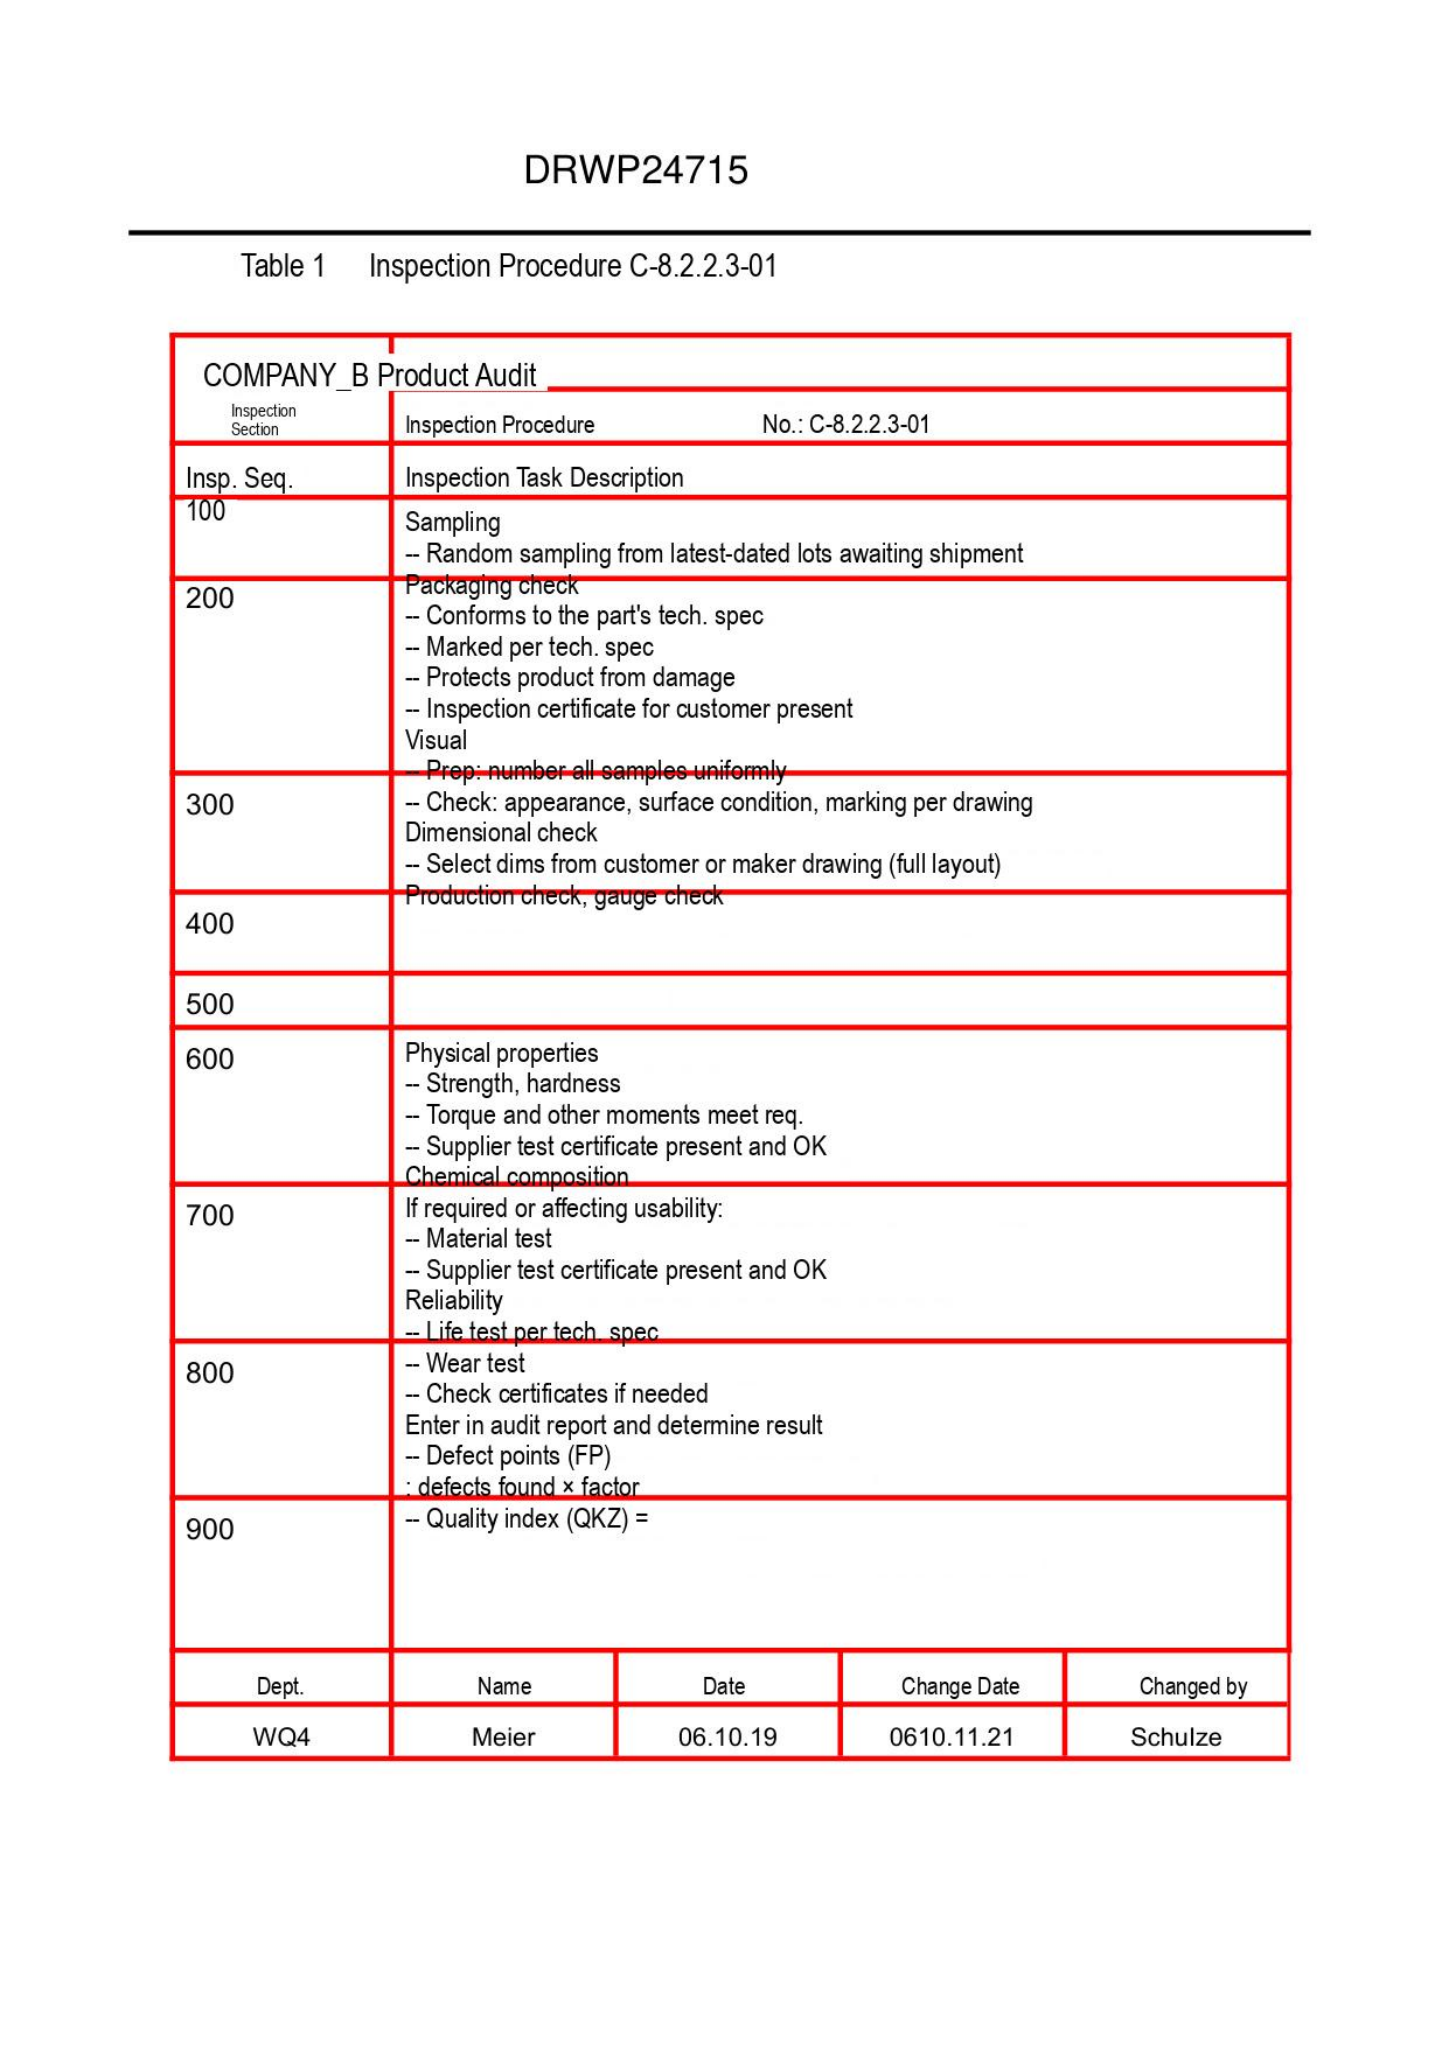DRWP24715

Table 1 Inspection Procedure C-8.2.2.3-01

COMPANY_B Product Audit

| Inspection Section | Inspection Procedure No.: C-8.2.2.3-01 |
|---|---|
| Insp. Seq. | Inspection Task Description |
| 100 | Sampling<br>-- Random sampling from latest-dated lots awaiting shipment |
| 200 | Packaging check<br>-- Conforms to the part's tech. spec<br>-- Marked per tech. spec<br>-- Protects product from damage<br>-- Inspection certificate for customer present<br>Visual<br>-- Prep: number all samples uniformly |
| 300 | -- Check: appearance, surface condition, marking per drawing<br>Dimensional check<br>-- Select dims from customer or maker drawing (full layout) |
| 400 | Production check, gauge check |
| 500 | |
| 600 | Physical properties<br>-- Strength, hardness<br>-- Torque and other moments meet req.<br>-- Supplier test certificate present and OK<br>Chemical composition |
| 700 | If required or affecting usability:<br>-- Material test<br>-- Supplier test certificate present and OK<br>Reliability<br>-- Life test per tech. spec |
| 800 | -- Wear test<br>-- Check certificates if needed<br>Enter in audit report and determine result<br>-- Defect points (FP)<br>: defects found × factor |
| 900 | -- Quality index (QKZ) = |

| Dept. | Name | Date | Change Date | Changed by |
|---|---|---|---|---|
| WQ4 | Meier | 06.10.19 | 0610.11.21 | Schulze |
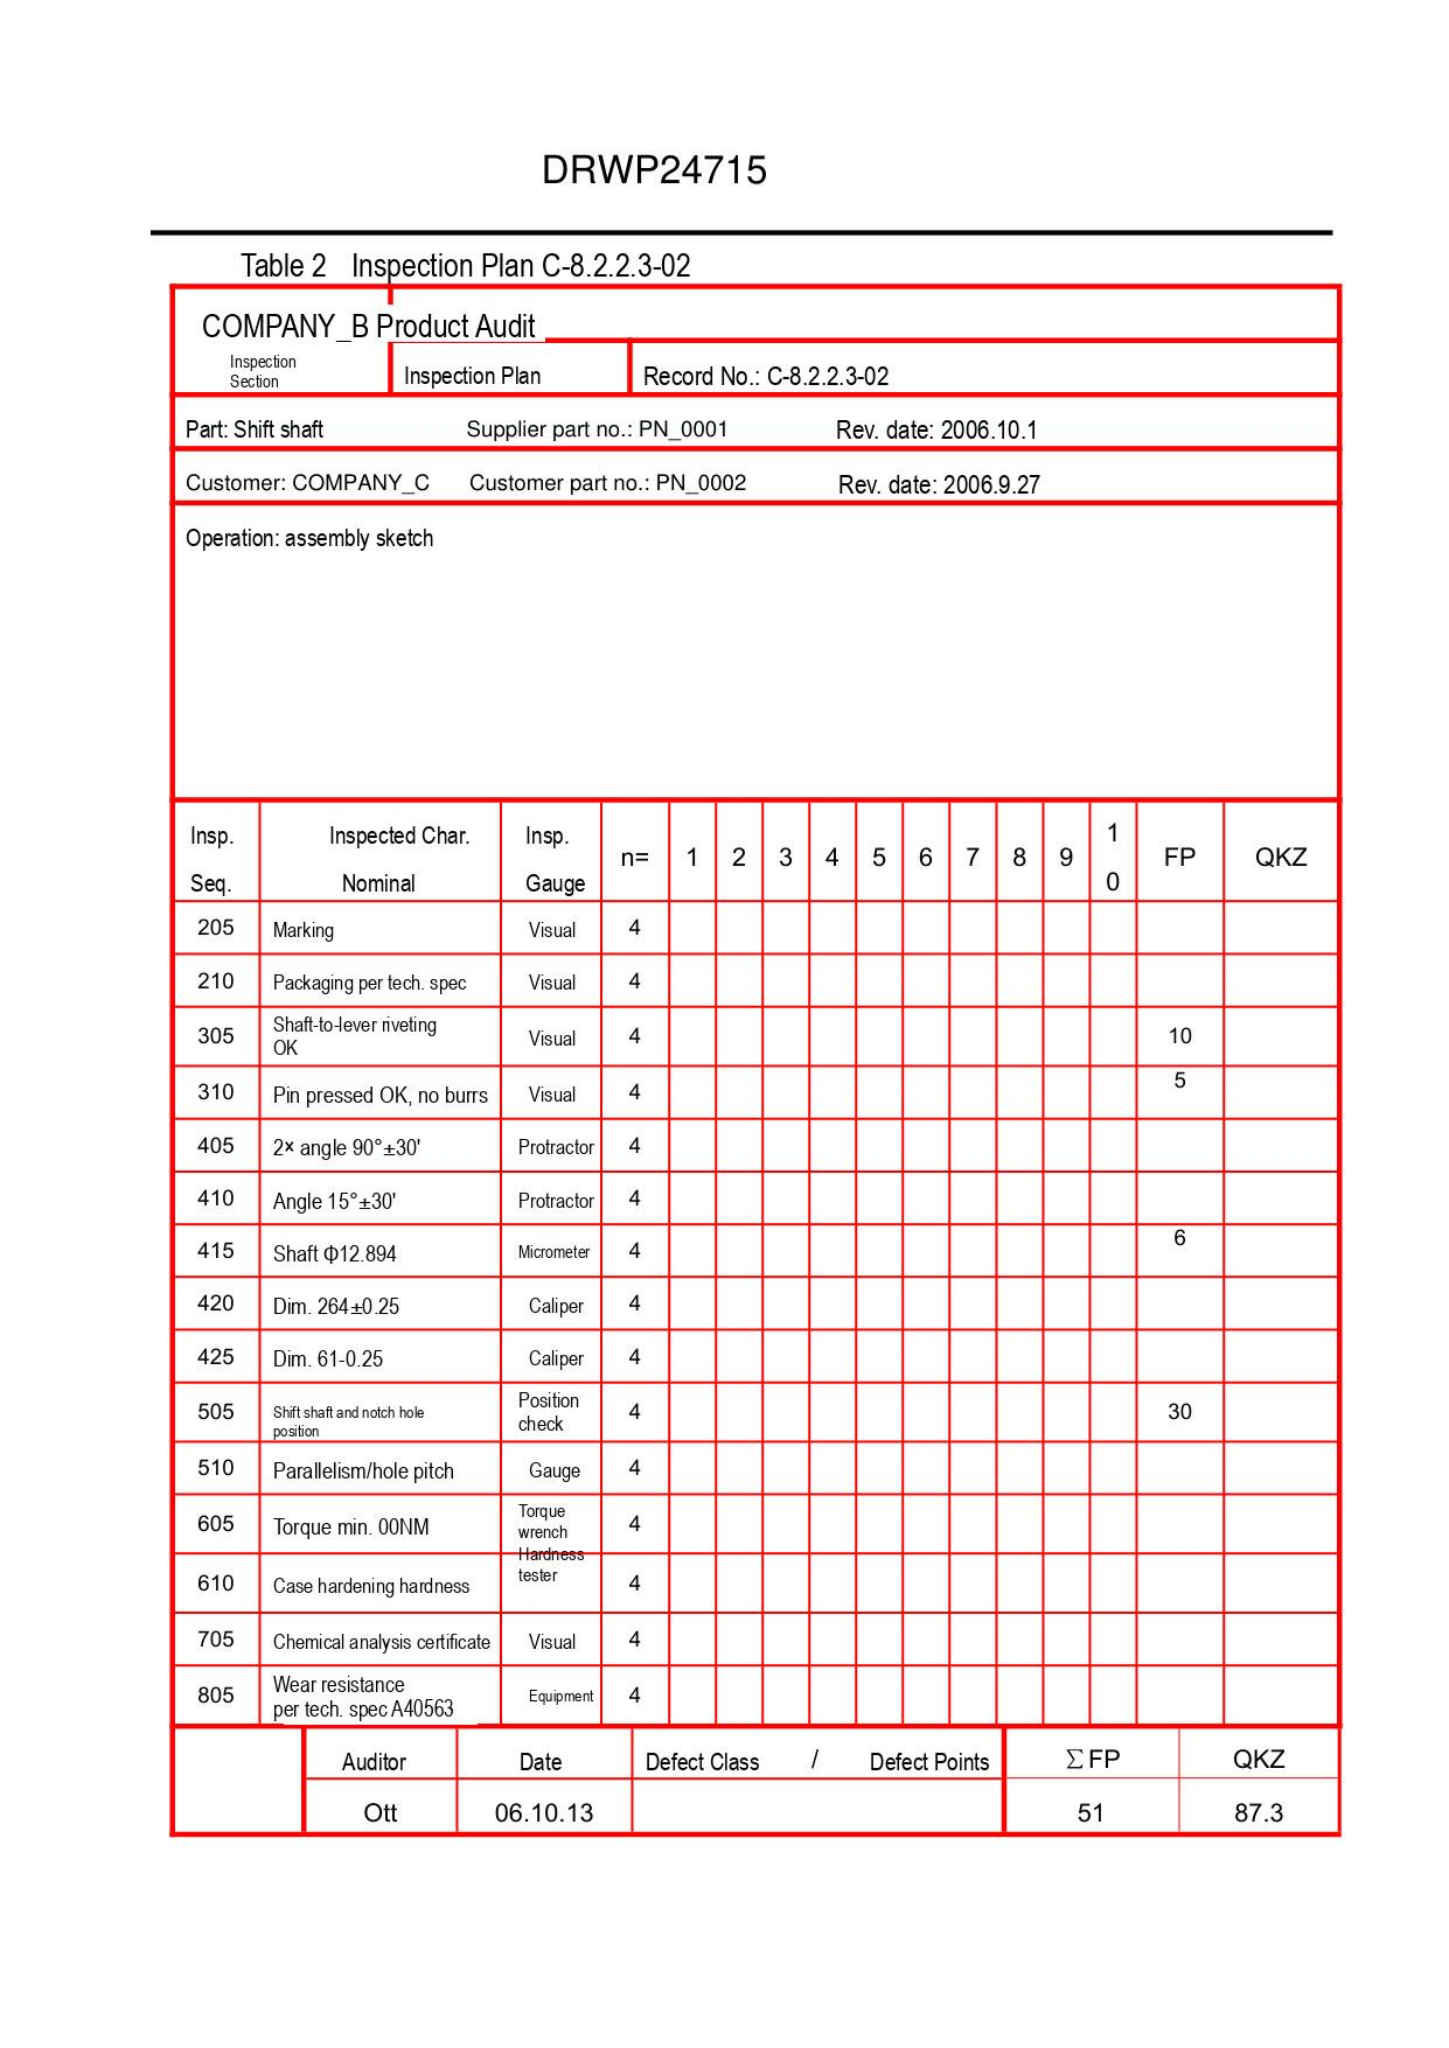DRWP24715

Table 2 Inspection Plan C-8.2.2.3-02

COMPANY_B Product Audit

Inspection Section | Inspection Plan | Record No.: C-8.2.2.3-02

Part: Shift shaft Supplier part no.: PN_0001 Rev. date: 2006.10.1

Customer: COMPANY_C Customer part no.: PN_0002 Rev. date: 2006.9.27

Operation: assembly sketch

| Insp. Seq. | Inspected Char. Nominal | Insp. Gauge | n= | 1 | 2 | 3 | 4 | 5 | 6 | 7 | 8 | 9 | 10 | FP | QKZ |
|---|---|---|---|---|---|---|---|---|---|---|---|---|---|---|---|
| 205 | Marking | Visual | 4 | | | | | | | | | | | | |
| 210 | Packaging per tech. spec | Visual | 4 | | | | | | | | | | | | |
| 305 | Shaft-to-lever riveting OK | Visual | 4 | | | | | | | | | | | 10 | |
| 310 | Pin pressed OK, no burrs | Visual | 4 | | | | | | | | | | | 5 | |
| 405 | 2× angle 90°±30' | Protractor | 4 | | | | | | | | | | | | |
| 410 | Angle 15°±30' | Protractor | 4 | | | | | | | | | | | | |
| 415 | Shaft Φ12.894 | Micrometer | 4 | | | | | | | | | | | 6 | |
| 420 | Dim. 264±0.25 | Caliper | 4 | | | | | | | | | | | | |
| 425 | Dim. 61-0.25 | Caliper | 4 | | | | | | | | | | | | |
| 505 | Shift shaft and notch hole position | Position check | 4 | | | | | | | | | | | 30 | |
| 510 | Parallelism/hole pitch | Gauge | 4 | | | | | | | | | | | | |
| 605 | Torque min. 00NM | Torque wrench | 4 | | | | | | | | | | | | |
| 610 | Case hardening hardness | Hardness tester | 4 | | | | | | | | | | | | |
| 705 | Chemical analysis certificate | Visual | 4 | | | | | | | | | | | | |
| 805 | Wear resistance per tech. spec A40563 | Equipment | 4 | | | | | | | | | | | | |

| | Auditor | Date | Defect Class / Defect Points | ΣFP | QKZ |
|---|---|---|---|---|---|
| | Ott | 06.10.13 | | 51 | 87.3 |
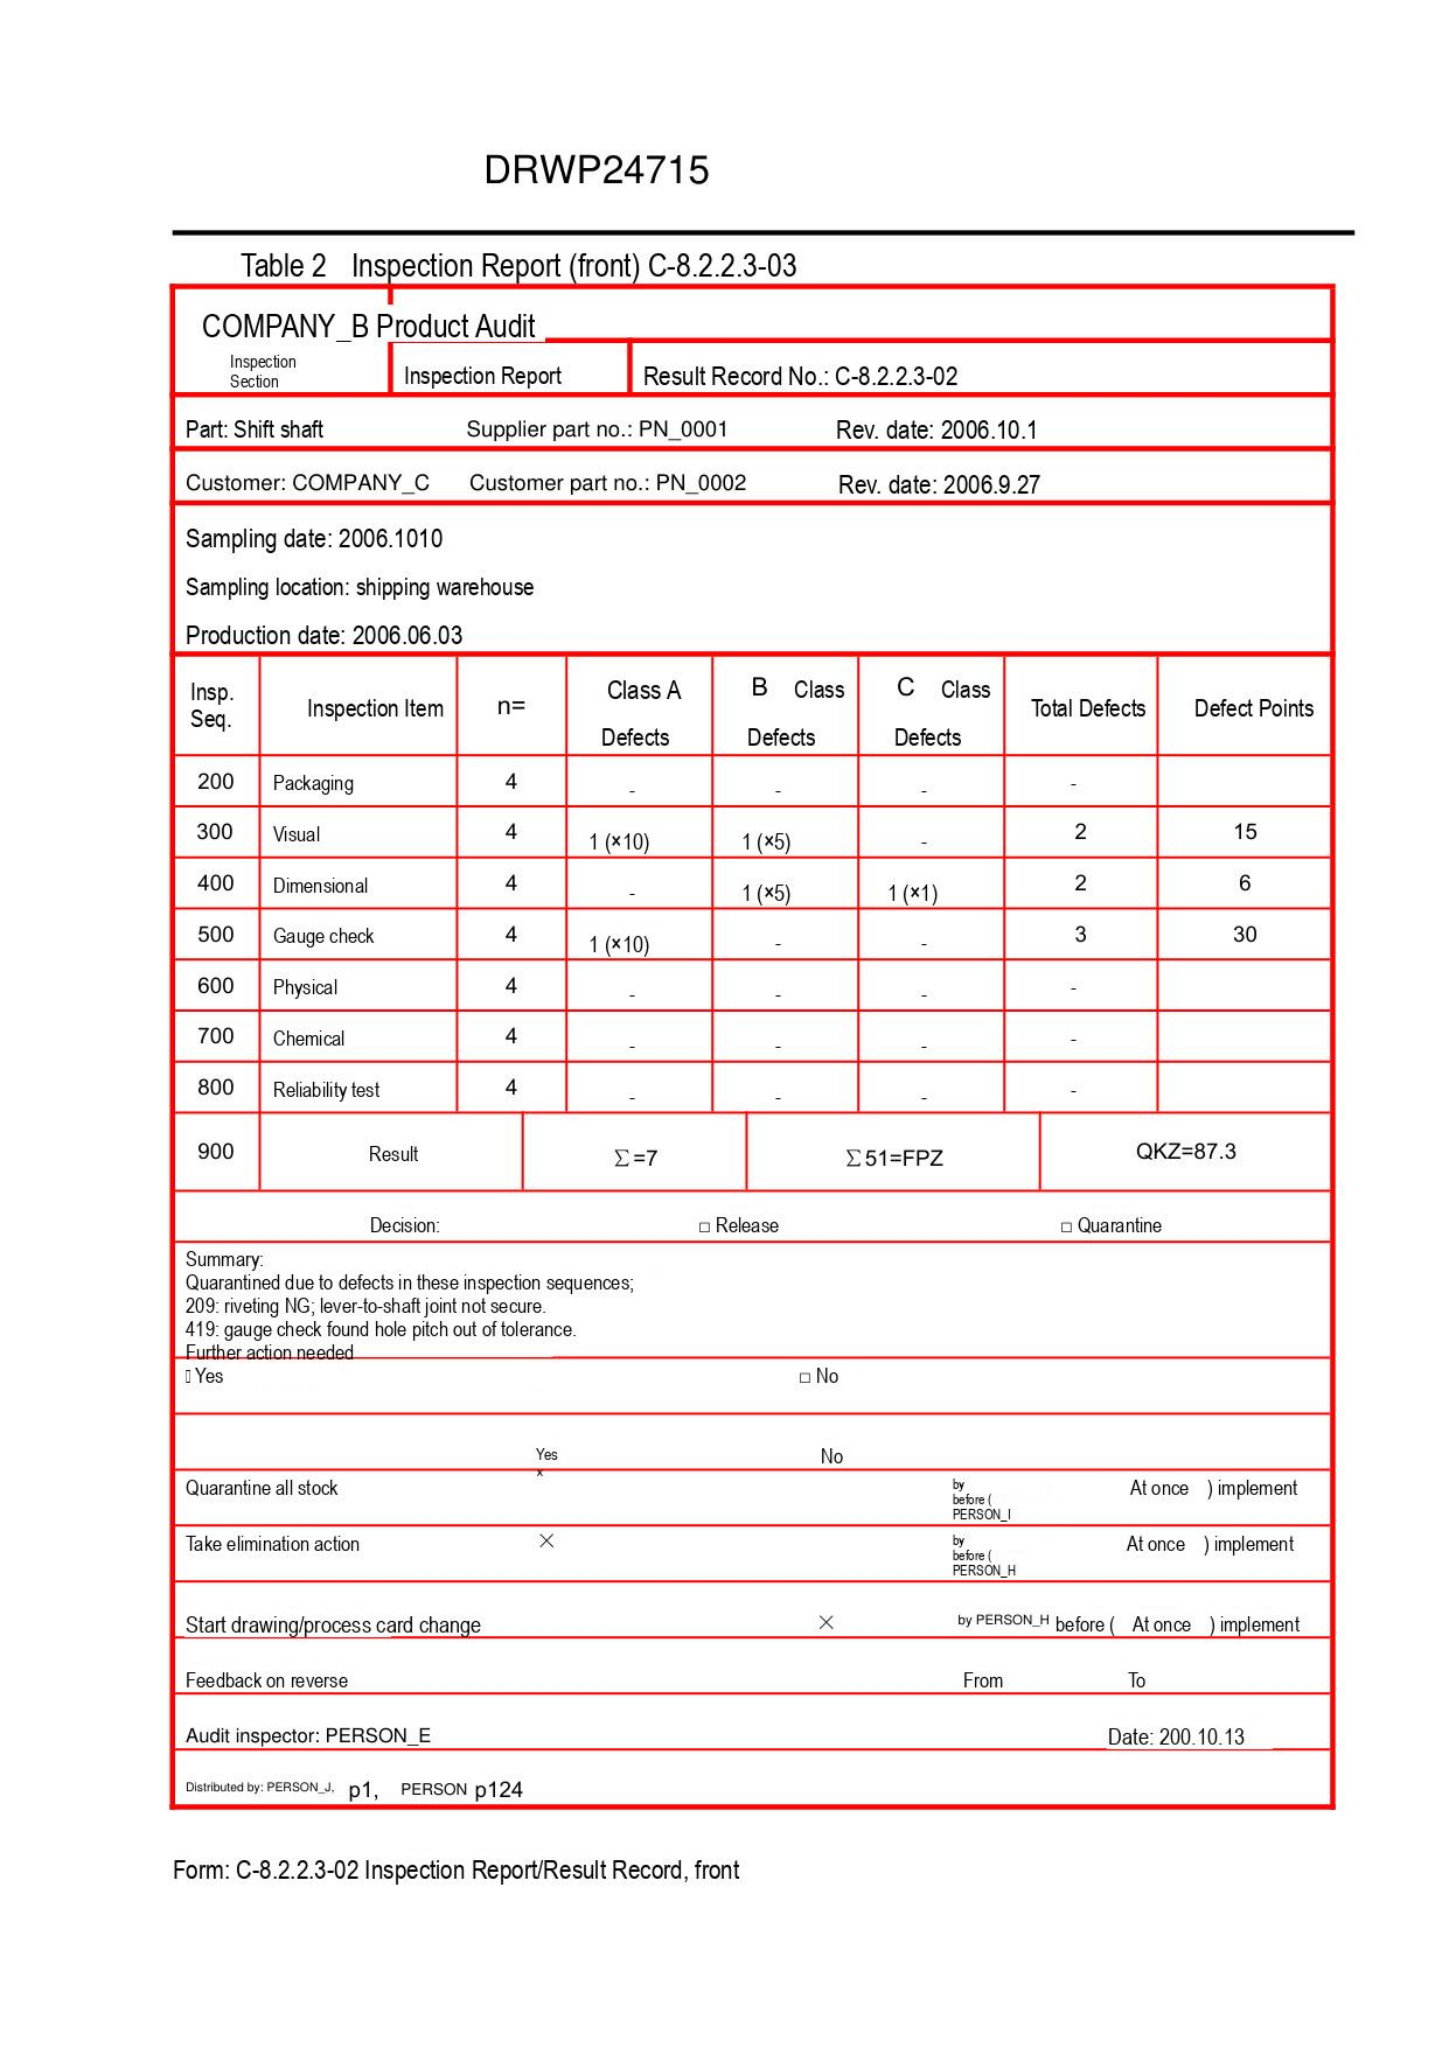DRWP24715

Table 2 Inspection Report (front) C-8.2.2.3-03

COMPANY_B Product Audit

Inspection Section | Inspection Report | Result Record No.: C-8.2.2.3-02

Part: Shift shaft  Supplier part no.: PN_0001  Rev. date: 2006.10.1

Customer: COMPANY_C  Customer part no.: PN_0002  Rev. date: 2006.9.27

Sampling date: 2006.1010

Sampling location: shipping warehouse

Production date: 2006.06.03

| Insp. Seq. | Inspection Item | n= | Class A Defects | B Class Defects | C Class Defects | Total Defects | Defect Points |
|---|---|---|---|---|---|---|---|
| 200 | Packaging | 4 | - | - | - | - | |
| 300 | Visual | 4 | 1 (×10) | 1 (×5) | - | 2 | 15 |
| 400 | Dimensional | 4 | - | 1 (×5) | 1 (×1) | 2 | 6 |
| 500 | Gauge check | 4 | 1 (×10) | - | - | 3 | 30 |
| 600 | Physical | 4 | - | - | - | - | |
| 700 | Chemical | 4 | - | - | - | - | |
| 800 | Reliability test | 4 | - | - | - | - | |
| 900 | Result | | Σ=7 | Σ51=FPZ | | QKZ=87.3 | |

Decision: □ Release □ Quarantine

Summary:
Quarantined due to defects in these inspection sequences;
209: riveting NG; lever-to-shaft joint not secure.
419: gauge check found hole pitch out of tolerance.
Further action needed
Yes □ No

| | Yes | No | | |
|---|---|---|---|---|
| Quarantine all stock | x | | by before ( PERSON_I | At once ) implement |
| Take elimination action | × | | by before ( PERSON_H | At once ) implement |
| Start drawing/process card change | | × | by PERSON_H before ( | At once ) implement |
| Feedback on reverse | | | From | To |

Audit inspector: PERSON_E  Date: 200.10.13

Distributed by: PERSON_J, p1, PERSON p124

Form: C-8.2.2.3-02 Inspection Report/Result Record, front
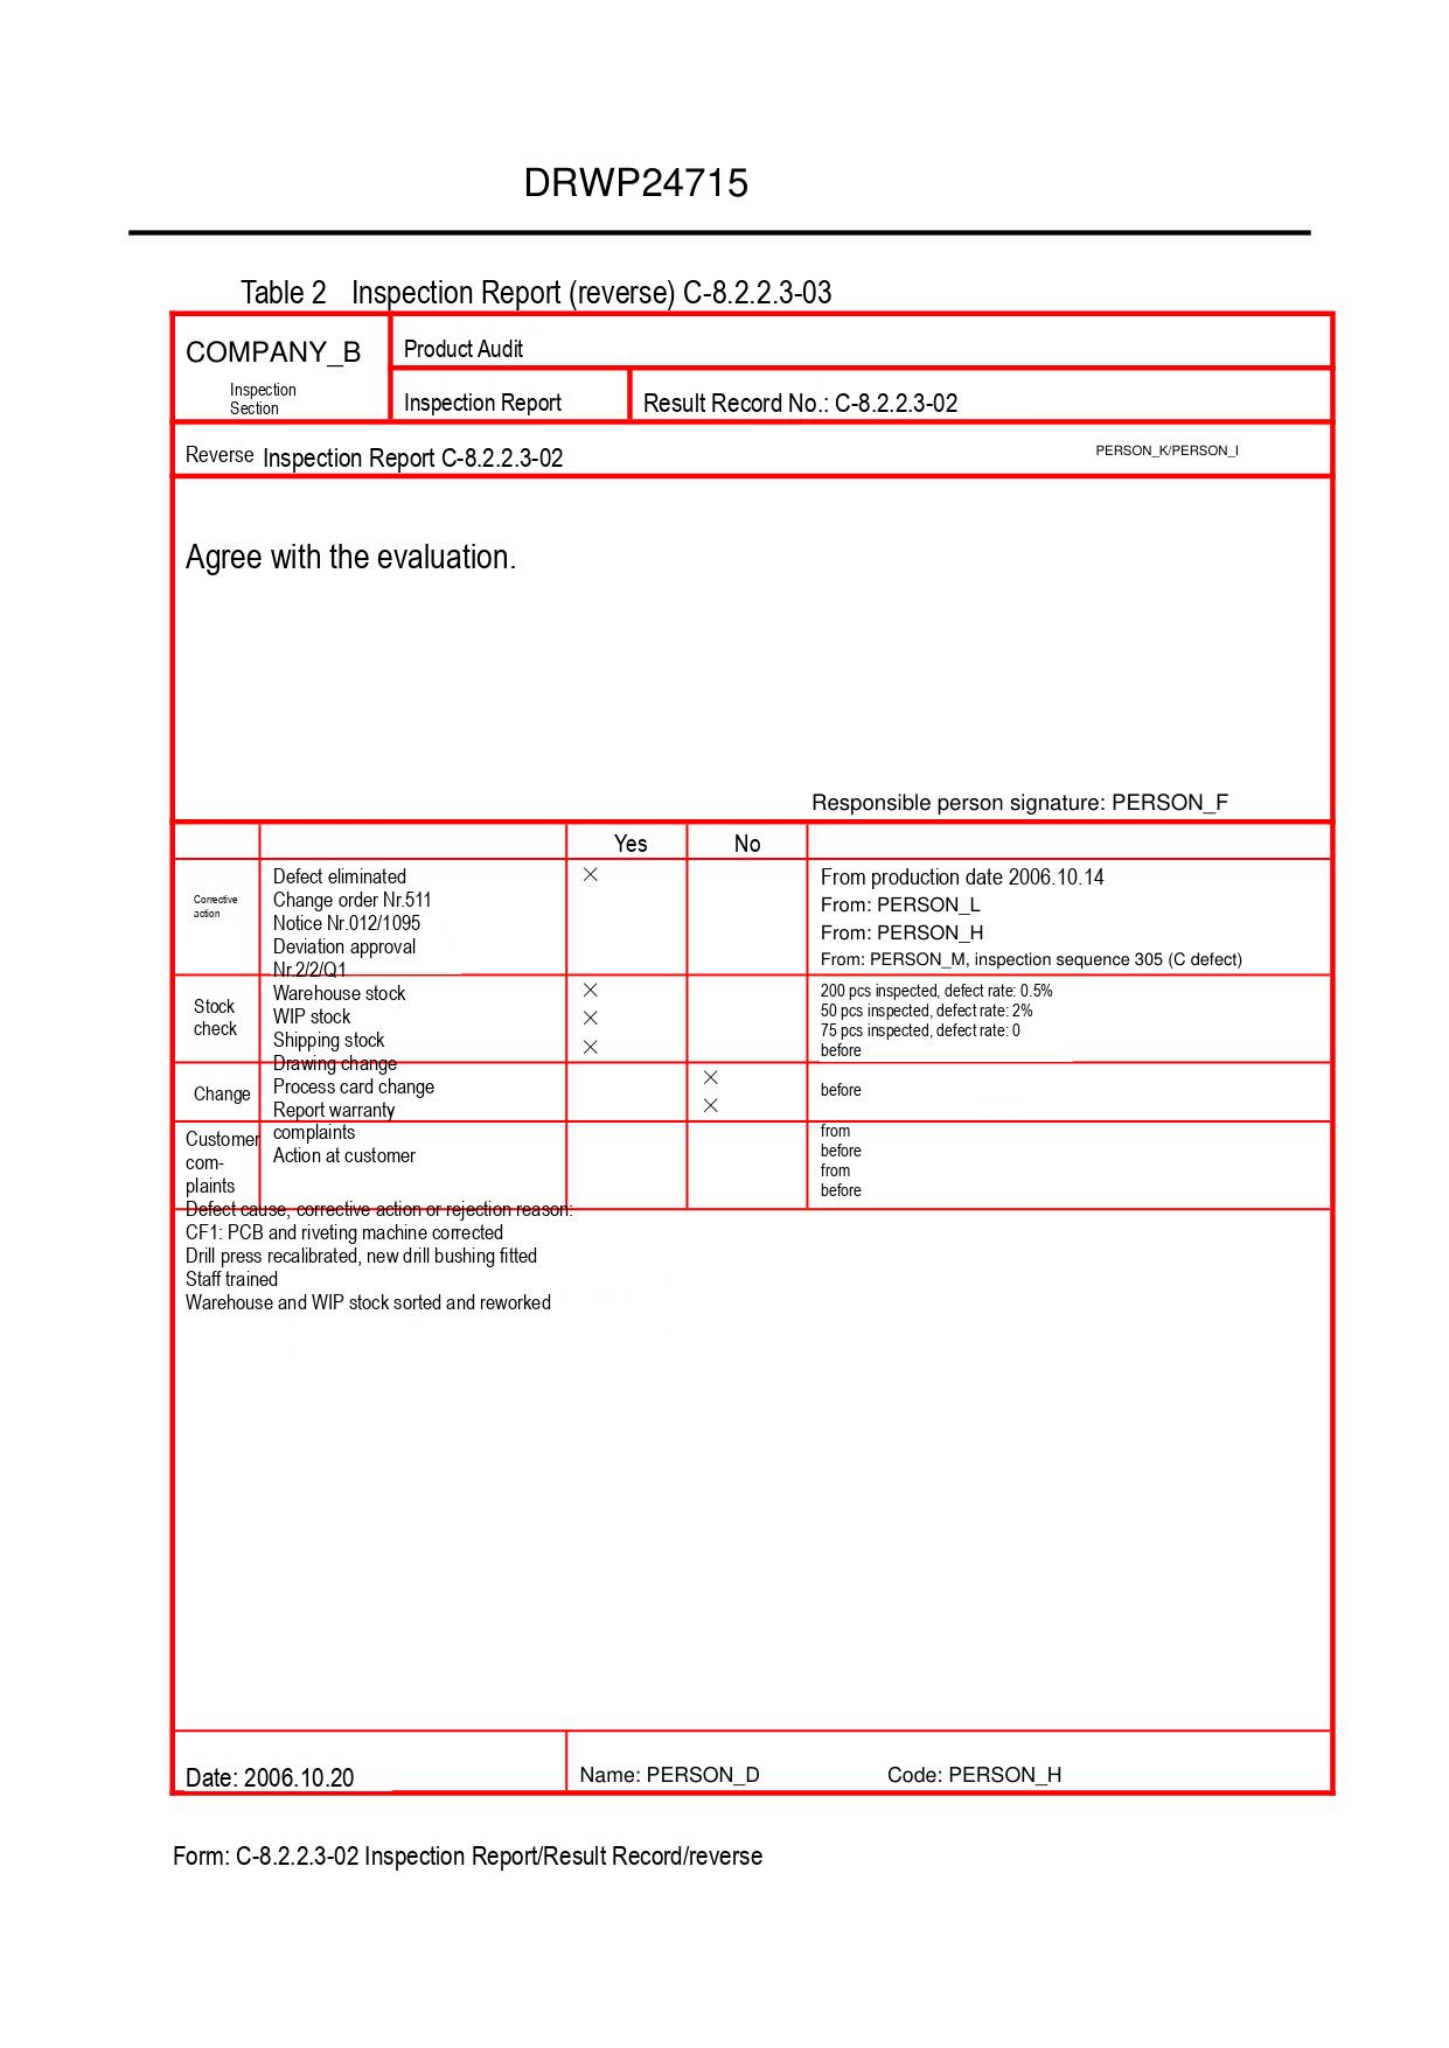DRWP24715

Table 2 Inspection Report (reverse) C-8.2.2.3-03

| COMPANY_B<br>Inspection Section | Product Audit | |
|---|---|---|
| | Inspection Report | Result Record No.: C-8.2.2.3-02 |

Reverse Inspection Report C-8.2.2.3-02 PERSON_K/PERSON_I

Agree with the evaluation.

Responsible person signature: PERSON_F

| | | Yes | No | |
|---|---|---|---|---|
| Corrective action | Defect eliminated<br>Change order Nr.511<br>Notice Nr.012/1095<br>Deviation approval Nr.2/2/Q1 | × | | From production date 2006.10.14<br>From: PERSON_L<br>From: PERSON_H<br>From: PERSON_M, inspection sequence 305 (C defect) |
| Stock check | Warehouse stock<br>WIP stock<br>Shipping stock | ×<br>×<br>× | | 200 pcs inspected, defect rate: 0.5%<br>50 pcs inspected, defect rate: 2%<br>75 pcs inspected, defect rate: 0<br>before |
| Change | Drawing change<br>Process card change<br>Report warranty | | ×<br>× | before |
| Customer com-plaints | complaints<br>Action at customer | | | from<br>before<br>from<br>before |

Defect cause, corrective action or rejection reason:
CF1: PCB and riveting machine corrected
Drill press recalibrated, new drill bushing fitted
Staff trained
Warehouse and WIP stock sorted and reworked

| Date: 2006.10.20 | Name: PERSON_D | Code: PERSON_H |
|---|---|---|

Form: C-8.2.2.3-02 Inspection Report/Result Record/reverse